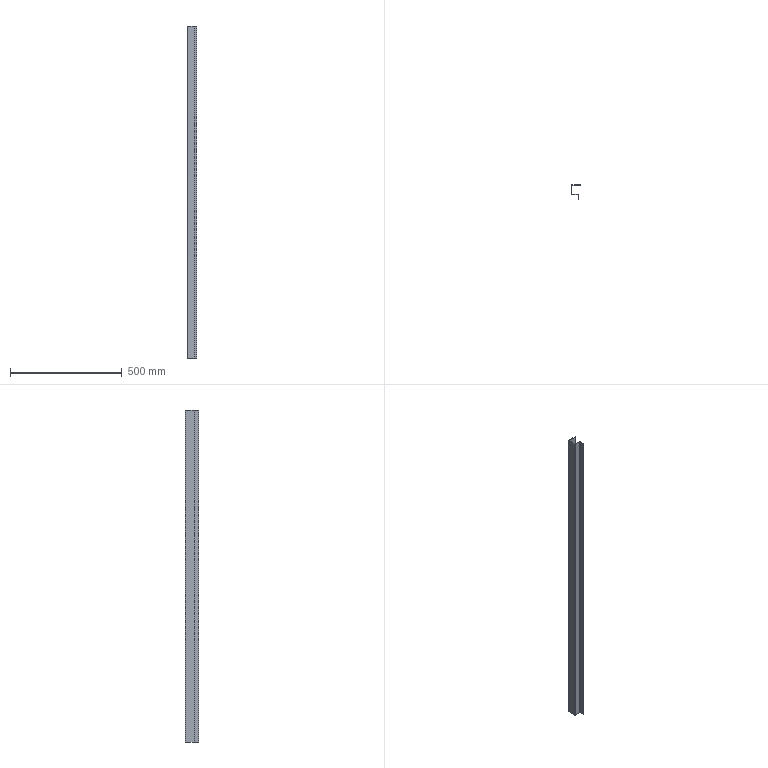Part | SolidWorks | features BaseBody 1 | 1 solid | 30 faces | box 41 x 61 x 1488 mm | volume 193542 mm3 | plane 24 | cylinder 6 | commonest cylinder face diameters 2 x3 4 x3
STEP:
#1=CARTESIAN_POINT('',(-10.,-42.,0.));
#2=VERTEX_POINT('',#1);
#3=CARTESIAN_POINT('',(-10.,-60.,0.));
#4=VERTEX_POINT('',#3);
#5=CARTESIAN_POINT('',(-10.,-40.,0.));
#6=DIRECTION('',(0.,-1.,0.));
#7=VECTOR('',#6,1000.);
#8=LINE('',#5,#7);
#9=EDGE_CURVE('',#2,#4,#8,.T.);
#10=ORIENTED_EDGE('',*,*,#9,.F.);
#11=CARTESIAN_POINT('',(-9.,-42.,0.));
#12=VERTEX_POINT('',#11);
#13=CARTESIAN_POINT('',(-10.,-42.,0.));
#14=DIRECTION('',(1.,0.,0.));
#15=VECTOR('',#14,1000.);
#16=LINE('',#13,#15);
#17=EDGE_CURVE('',#2,#12,#16,.T.);
#18=ORIENTED_EDGE('',*,*,#17,.T.);
#19=CARTESIAN_POINT('',(-9.,-60.,0.));
#20=VERTEX_POINT('',#19);
#21=CARTESIAN_POINT('',(-9.,-40.,0.));
#22=DIRECTION('',(0.,-1.,0.));
#23=VECTOR('',#22,1000.);
#24=LINE('',#21,#23);
#25=EDGE_CURVE('',#12,#20,#24,.T.);
#26=ORIENTED_EDGE('',*,*,#25,.T.);
#27=CARTESIAN_POINT('',(-9.,-60.,0.));
#28=DIRECTION('',(-1.,0.,0.));
#29=VECTOR('',#28,1000.);
#30=LINE('',#27,#29);
#31=EDGE_CURVE('',#20,#4,#30,.T.);
#32=ORIENTED_EDGE('',*,*,#31,.T.);
#33=EDGE_LOOP('',(#10,#18,#26,#32));
#34=FACE_OUTER_BOUND('',#33,.T.);
#35=CARTESIAN_POINT('',(-11.,-42.,0.));
#36=DIRECTION('',(0.,0.,1.));
#37=DIRECTION('',(1.,0.,0.));
#38=AXIS2_PLACEMENT_3D('',#35,#36,#37);
#39=PLANE('',#38);
#40=ADVANCED_FACE('',(#34),#39,.F.);
#41=CARTESIAN_POINT('',(0.,1.,1488.));
#42=VERTEX_POINT('',#41);
#43=CARTESIAN_POINT('',(-39.,1.,1488.));
#44=VERTEX_POINT('',#43);
#45=CARTESIAN_POINT('',(0.,1.,1488.));
#46=DIRECTION('',(-1.,0.,0.));
#47=VECTOR('',#46,1000.);
#48=LINE('',#45,#47);
#49=EDGE_CURVE('',#42,#44,#48,.T.);
#50=ORIENTED_EDGE('',*,*,#49,.T.);
#51=CARTESIAN_POINT('',(-39.,0.,1488.));
#52=VERTEX_POINT('',#51);
#53=CARTESIAN_POINT('',(-39.,1.,1488.));
#54=DIRECTION('',(0.,-1.,0.));
#55=VECTOR('',#54,1000.);
#56=LINE('',#53,#55);
#57=EDGE_CURVE('',#44,#52,#56,.T.);
#58=ORIENTED_EDGE('',*,*,#57,.T.);
#59=CARTESIAN_POINT('',(0.,0.,1488.));
#60=VERTEX_POINT('',#59);
#61=CARTESIAN_POINT('',(0.,0.,1488.));
#62=DIRECTION('',(-1.,0.,0.));
#63=VECTOR('',#62,1000.);
#64=LINE('',#61,#63);
#65=EDGE_CURVE('',#60,#52,#64,.T.);
#66=ORIENTED_EDGE('',*,*,#65,.F.);
#67=CARTESIAN_POINT('',(0.,1.,1488.));
#68=DIRECTION('',(0.,-1.,0.));
#69=VECTOR('',#68,1000.);
#70=LINE('',#67,#69);
#71=EDGE_CURVE('',#42,#60,#70,.T.);
#72=ORIENTED_EDGE('',*,*,#71,.F.);
#73=EDGE_LOOP('',(#50,#58,#66,#72));
#74=FACE_OUTER_BOUND('',#73,.T.);
#75=CARTESIAN_POINT('',(-11.,-42.,1488.));
#76=DIRECTION('',(0.,0.,1.));
#77=DIRECTION('',(1.,0.,0.));
#78=AXIS2_PLACEMENT_3D('',#75,#76,#77);
#79=PLANE('',#78);
#80=ADVANCED_FACE('',(#74),#79,.T.);
#81=CARTESIAN_POINT('',(-11.,-41.,0.));
#82=VERTEX_POINT('',#81);
#83=CARTESIAN_POINT('',(-11.,-42.,0.));
#84=DIRECTION('',(0.,0.,-1.));
#85=DIRECTION('',(1.,0.,0.));
#86=AXIS2_PLACEMENT_3D('',#83,#84,#85);
#87=CIRCLE('',#86,1.);
#88=EDGE_CURVE('',#82,#2,#87,.T.);
#89=ORIENTED_EDGE('',*,*,#88,.T.);
#90=CARTESIAN_POINT('',(-10.,-42.,1488.));
#91=VERTEX_POINT('',#90);
#92=CARTESIAN_POINT('',(-10.,-42.,1488.));
#93=DIRECTION('',(0.,0.,-1.));
#94=VECTOR('',#93,1000.);
#95=LINE('',#92,#94);
#96=EDGE_CURVE('',#91,#2,#95,.T.);
#97=ORIENTED_EDGE('',*,*,#96,.F.);
#98=CARTESIAN_POINT('',(-11.,-41.,1488.));
#99=VERTEX_POINT('',#98);
#100=CARTESIAN_POINT('',(-11.,-42.,1488.));
#101=DIRECTION('',(0.,0.,-1.));
#102=DIRECTION('',(1.,0.,0.));
#103=AXIS2_PLACEMENT_3D('',#100,#101,#102);
#104=CIRCLE('',#103,1.);
#105=EDGE_CURVE('',#99,#91,#104,.T.);
#106=ORIENTED_EDGE('',*,*,#105,.F.);
#107=CARTESIAN_POINT('',(-11.,-41.,1488.));
#108=DIRECTION('',(0.,0.,-1.));
#109=VECTOR('',#108,1000.);
#110=LINE('',#107,#109);
#111=EDGE_CURVE('',#99,#82,#110,.T.);
#112=ORIENTED_EDGE('',*,*,#111,.T.);
#113=EDGE_LOOP('',(#89,#97,#106,#112));
#114=FACE_OUTER_BOUND('',#113,.T.);
#115=CARTESIAN_POINT('',(-11.,-42.,1488.));
#116=DIRECTION('',(0.,0.,-1.));
#117=DIRECTION('',(-1.,0.,0.));
#118=AXIS2_PLACEMENT_3D('',#115,#116,#117);
#119=CYLINDRICAL_SURFACE('',#118,1.);
#120=ADVANCED_FACE('',(#114),#119,.F.);
#121=CARTESIAN_POINT('',(-39.,-41.,0.));
#122=VERTEX_POINT('',#121);
#123=CARTESIAN_POINT('',(-40.,-41.,0.));
#124=DIRECTION('',(1.,0.,0.));
#125=VECTOR('',#124,1000.);
#126=LINE('',#123,#125);
#127=EDGE_CURVE('',#122,#82,#126,.T.);
#128=ORIENTED_EDGE('',*,*,#127,.T.);
#129=ORIENTED_EDGE('',*,*,#111,.F.);
#130=CARTESIAN_POINT('',(-39.,-41.,1488.));
#131=VERTEX_POINT('',#130);
#132=CARTESIAN_POINT('',(-40.,-41.,1488.));
#133=DIRECTION('',(1.,0.,0.));
#134=VECTOR('',#133,1000.);
#135=LINE('',#132,#134);
#136=EDGE_CURVE('',#131,#99,#135,.T.);
#137=ORIENTED_EDGE('',*,*,#136,.F.);
#138=CARTESIAN_POINT('',(-39.,-41.,1488.));
#139=DIRECTION('',(0.,0.,-1.));
#140=VECTOR('',#139,1000.);
#141=LINE('',#138,#140);
#142=EDGE_CURVE('',#131,#122,#141,.T.);
#143=ORIENTED_EDGE('',*,*,#142,.T.);
#144=EDGE_LOOP('',(#128,#129,#137,#143));
#145=FACE_OUTER_BOUND('',#144,.T.);
#146=CARTESIAN_POINT('',(-40.,-41.,1488.));
#147=DIRECTION('',(0.,1.,0.));
#148=DIRECTION('',(1.,0.,0.));
#149=AXIS2_PLACEMENT_3D('',#146,#147,#148);
#150=PLANE('',#149);
#151=ADVANCED_FACE('',(#145),#150,.F.);
#152=CARTESIAN_POINT('',(-41.,-39.,0.));
#153=VERTEX_POINT('',#152);
#154=CARTESIAN_POINT('',(-39.,-39.,0.));
#155=DIRECTION('',(0.,0.,1.));
#156=DIRECTION('',(1.,0.,0.));
#157=AXIS2_PLACEMENT_3D('',#154,#155,#156);
#158=CIRCLE('',#157,2.);
#159=EDGE_CURVE('',#153,#122,#158,.T.);
#160=ORIENTED_EDGE('',*,*,#159,.T.);
#161=ORIENTED_EDGE('',*,*,#142,.F.);
#162=CARTESIAN_POINT('',(-41.,-39.,1488.));
#163=VERTEX_POINT('',#162);
#164=CARTESIAN_POINT('',(-39.,-39.,1488.));
#165=DIRECTION('',(0.,0.,1.));
#166=DIRECTION('',(1.,0.,0.));
#167=AXIS2_PLACEMENT_3D('',#164,#165,#166);
#168=CIRCLE('',#167,2.);
#169=EDGE_CURVE('',#163,#131,#168,.T.);
#170=ORIENTED_EDGE('',*,*,#169,.F.);
#171=CARTESIAN_POINT('',(-41.,-39.,1488.));
#172=DIRECTION('',(0.,0.,-1.));
#173=VECTOR('',#172,1000.);
#174=LINE('',#171,#173);
#175=EDGE_CURVE('',#163,#153,#174,.T.);
#176=ORIENTED_EDGE('',*,*,#175,.T.);
#177=EDGE_LOOP('',(#160,#161,#170,#176));
#178=FACE_OUTER_BOUND('',#177,.T.);
#179=CARTESIAN_POINT('',(-39.,-39.,1488.));
#180=DIRECTION('',(0.,0.,-1.));
#181=DIRECTION('',(-1.,0.,0.));
#182=AXIS2_PLACEMENT_3D('',#179,#180,#181);
#183=CYLINDRICAL_SURFACE('',#182,2.);
#184=ADVANCED_FACE('',(#178),#183,.T.);
#185=CARTESIAN_POINT('',(-41.,-1.,0.));
#186=VERTEX_POINT('',#185);
#187=CARTESIAN_POINT('',(-41.,0.,0.));
#188=DIRECTION('',(0.,-1.,0.));
#189=VECTOR('',#188,1000.);
#190=LINE('',#187,#189);
#191=EDGE_CURVE('',#186,#153,#190,.T.);
#192=ORIENTED_EDGE('',*,*,#191,.T.);
#193=ORIENTED_EDGE('',*,*,#175,.F.);
#194=CARTESIAN_POINT('',(-41.,-1.,1488.));
#195=VERTEX_POINT('',#194);
#196=CARTESIAN_POINT('',(-41.,0.,1488.));
#197=DIRECTION('',(0.,-1.,0.));
#198=VECTOR('',#197,1000.);
#199=LINE('',#196,#198);
#200=EDGE_CURVE('',#195,#163,#199,.T.);
#201=ORIENTED_EDGE('',*,*,#200,.F.);
#202=CARTESIAN_POINT('',(-41.,-1.,1488.));
#203=DIRECTION('',(0.,0.,-1.));
#204=VECTOR('',#203,1000.);
#205=LINE('',#202,#204);
#206=EDGE_CURVE('',#195,#186,#205,.T.);
#207=ORIENTED_EDGE('',*,*,#206,.T.);
#208=EDGE_LOOP('',(#192,#193,#201,#207));
#209=FACE_OUTER_BOUND('',#208,.T.);
#210=CARTESIAN_POINT('',(-41.,0.,1488.));
#211=DIRECTION('',(1.,0.,0.));
#212=DIRECTION('',(0.,1.,0.));
#213=AXIS2_PLACEMENT_3D('',#210,#211,#212);
#214=PLANE('',#213);
#215=ADVANCED_FACE('',(#209),#214,.F.);
#216=CARTESIAN_POINT('',(-39.,1.,0.));
#217=VERTEX_POINT('',#216);
#218=CARTESIAN_POINT('',(-39.,-1.,0.));
#219=DIRECTION('',(0.,0.,1.));
#220=DIRECTION('',(1.,0.,0.));
#221=AXIS2_PLACEMENT_3D('',#218,#219,#220);
#222=CIRCLE('',#221,2.);
#223=EDGE_CURVE('',#217,#186,#222,.T.);
#224=ORIENTED_EDGE('',*,*,#223,.T.);
#225=ORIENTED_EDGE('',*,*,#206,.F.);
#226=CARTESIAN_POINT('',(-39.,-1.,1488.));
#227=DIRECTION('',(0.,0.,1.));
#228=DIRECTION('',(1.,0.,0.));
#229=AXIS2_PLACEMENT_3D('',#226,#227,#228);
#230=CIRCLE('',#229,2.);
#231=EDGE_CURVE('',#44,#195,#230,.T.);
#232=ORIENTED_EDGE('',*,*,#231,.F.);
#233=CARTESIAN_POINT('',(-39.,1.,1488.));
#234=DIRECTION('',(0.,0.,-1.));
#235=VECTOR('',#234,1000.);
#236=LINE('',#233,#235);
#237=EDGE_CURVE('',#44,#217,#236,.T.);
#238=ORIENTED_EDGE('',*,*,#237,.T.);
#239=EDGE_LOOP('',(#224,#225,#232,#238));
#240=FACE_OUTER_BOUND('',#239,.T.);
#241=CARTESIAN_POINT('',(-39.,-1.,1488.));
#242=DIRECTION('',(0.,0.,-1.));
#243=DIRECTION('',(-1.,0.,0.));
#244=AXIS2_PLACEMENT_3D('',#241,#242,#243);
#245=CYLINDRICAL_SURFACE('',#244,2.);
#246=ADVANCED_FACE('',(#240),#245,.T.);
#247=CARTESIAN_POINT('',(0.,1.,0.));
#248=VERTEX_POINT('',#247);
#249=CARTESIAN_POINT('',(0.,1.,0.));
#250=DIRECTION('',(-1.,0.,0.));
#251=VECTOR('',#250,1000.);
#252=LINE('',#249,#251);
#253=EDGE_CURVE('',#248,#217,#252,.T.);
#254=ORIENTED_EDGE('',*,*,#253,.T.);
#255=ORIENTED_EDGE('',*,*,#237,.F.);
#256=ORIENTED_EDGE('',*,*,#49,.F.);
#257=CARTESIAN_POINT('',(0.,1.,1488.));
#258=DIRECTION('',(0.,0.,-1.));
#259=VECTOR('',#258,1000.);
#260=LINE('',#257,#259);
#261=EDGE_CURVE('',#42,#248,#260,.T.);
#262=ORIENTED_EDGE('',*,*,#261,.T.);
#263=EDGE_LOOP('',(#254,#255,#256,#262));
#264=FACE_OUTER_BOUND('',#263,.T.);
#265=CARTESIAN_POINT('',(0.,1.,1488.));
#266=DIRECTION('',(0.,-1.,0.));
#267=DIRECTION('',(0.,0.,-1.));
#268=AXIS2_PLACEMENT_3D('',#265,#266,#267);
#269=PLANE('',#268);
#270=ADVANCED_FACE('',(#264),#269,.F.);
#271=CARTESIAN_POINT('',(0.,0.,0.));
#272=VERTEX_POINT('',#271);
#273=CARTESIAN_POINT('',(0.,1.,0.));
#274=DIRECTION('',(0.,-1.,0.));
#275=VECTOR('',#274,1000.);
#276=LINE('',#273,#275);
#277=EDGE_CURVE('',#248,#272,#276,.T.);
#278=ORIENTED_EDGE('',*,*,#277,.F.);
#279=ORIENTED_EDGE('',*,*,#261,.F.);
#280=ORIENTED_EDGE('',*,*,#71,.T.);
#281=CARTESIAN_POINT('',(0.,0.,1488.));
#282=DIRECTION('',(0.,0.,-1.));
#283=VECTOR('',#282,1000.);
#284=LINE('',#281,#283);
#285=EDGE_CURVE('',#60,#272,#284,.T.);
#286=ORIENTED_EDGE('',*,*,#285,.T.);
#287=EDGE_LOOP('',(#278,#279,#280,#286));
#288=FACE_OUTER_BOUND('',#287,.T.);
#289=CARTESIAN_POINT('',(0.,1.,1488.));
#290=DIRECTION('',(1.,0.,0.));
#291=DIRECTION('',(0.,1.,0.));
#292=AXIS2_PLACEMENT_3D('',#289,#290,#291);
#293=PLANE('',#292);
#294=ADVANCED_FACE('',(#288),#293,.T.);
#295=CARTESIAN_POINT('',(-39.,0.,0.));
#296=VERTEX_POINT('',#295);
#297=CARTESIAN_POINT('',(0.,0.,0.));
#298=DIRECTION('',(-1.,0.,0.));
#299=VECTOR('',#298,1000.);
#300=LINE('',#297,#299);
#301=EDGE_CURVE('',#272,#296,#300,.T.);
#302=ORIENTED_EDGE('',*,*,#301,.F.);
#303=ORIENTED_EDGE('',*,*,#285,.F.);
#304=ORIENTED_EDGE('',*,*,#65,.T.);
#305=CARTESIAN_POINT('',(-39.,0.,1488.));
#306=DIRECTION('',(0.,0.,-1.));
#307=VECTOR('',#306,1000.);
#308=LINE('',#305,#307);
#309=EDGE_CURVE('',#52,#296,#308,.T.);
#310=ORIENTED_EDGE('',*,*,#309,.T.);
#311=EDGE_LOOP('',(#302,#303,#304,#310));
#312=FACE_OUTER_BOUND('',#311,.T.);
#313=CARTESIAN_POINT('',(0.,0.,1488.));
#314=DIRECTION('',(0.,-1.,0.));
#315=DIRECTION('',(0.,0.,-1.));
#316=AXIS2_PLACEMENT_3D('',#313,#314,#315);
#317=PLANE('',#316);
#318=ADVANCED_FACE('',(#312),#317,.T.);
#319=CARTESIAN_POINT('',(-40.,-1.,0.));
#320=VERTEX_POINT('',#319);
#321=CARTESIAN_POINT('',(-39.,-1.,0.));
#322=DIRECTION('',(0.,0.,1.));
#323=DIRECTION('',(-1.,0.,0.));
#324=AXIS2_PLACEMENT_3D('',#321,#322,#323);
#325=CIRCLE('',#324,1.);
#326=EDGE_CURVE('',#296,#320,#325,.T.);
#327=ORIENTED_EDGE('',*,*,#326,.F.);
#328=ORIENTED_EDGE('',*,*,#309,.F.);
#329=CARTESIAN_POINT('',(-40.,-1.,1488.));
#330=VERTEX_POINT('',#329);
#331=CARTESIAN_POINT('',(-39.,-1.,1488.));
#332=DIRECTION('',(0.,0.,1.));
#333=DIRECTION('',(-1.,0.,0.));
#334=AXIS2_PLACEMENT_3D('',#331,#332,#333);
#335=CIRCLE('',#334,1.);
#336=EDGE_CURVE('',#52,#330,#335,.T.);
#337=ORIENTED_EDGE('',*,*,#336,.T.);
#338=CARTESIAN_POINT('',(-40.,-1.,1488.));
#339=DIRECTION('',(0.,0.,-1.));
#340=VECTOR('',#339,1000.);
#341=LINE('',#338,#340);
#342=EDGE_CURVE('',#330,#320,#341,.T.);
#343=ORIENTED_EDGE('',*,*,#342,.T.);
#344=EDGE_LOOP('',(#327,#328,#337,#343));
#345=FACE_OUTER_BOUND('',#344,.T.);
#346=CARTESIAN_POINT('',(-39.,-1.,1488.));
#347=DIRECTION('',(0.,0.,-1.));
#348=DIRECTION('',(-1.,0.,0.));
#349=AXIS2_PLACEMENT_3D('',#346,#347,#348);
#350=CYLINDRICAL_SURFACE('',#349,1.);
#351=ADVANCED_FACE('',(#345),#350,.F.);
#352=CARTESIAN_POINT('',(-40.,-39.,0.));
#353=VERTEX_POINT('',#352);
#354=CARTESIAN_POINT('',(-40.,0.,0.));
#355=DIRECTION('',(0.,-1.,0.));
#356=VECTOR('',#355,1000.);
#357=LINE('',#354,#356);
#358=EDGE_CURVE('',#320,#353,#357,.T.);
#359=ORIENTED_EDGE('',*,*,#358,.F.);
#360=ORIENTED_EDGE('',*,*,#342,.F.);
#361=CARTESIAN_POINT('',(-40.,-39.,1488.));
#362=VERTEX_POINT('',#361);
#363=CARTESIAN_POINT('',(-40.,0.,1488.));
#364=DIRECTION('',(0.,-1.,0.));
#365=VECTOR('',#364,1000.);
#366=LINE('',#363,#365);
#367=EDGE_CURVE('',#330,#362,#366,.T.);
#368=ORIENTED_EDGE('',*,*,#367,.T.);
#369=CARTESIAN_POINT('',(-40.,-39.,1488.));
#370=DIRECTION('',(0.,0.,-1.));
#371=VECTOR('',#370,1000.);
#372=LINE('',#369,#371);
#373=EDGE_CURVE('',#362,#353,#372,.T.);
#374=ORIENTED_EDGE('',*,*,#373,.T.);
#375=EDGE_LOOP('',(#359,#360,#368,#374));
#376=FACE_OUTER_BOUND('',#375,.T.);
#377=CARTESIAN_POINT('',(-40.,0.,1488.));
#378=DIRECTION('',(1.,0.,0.));
#379=DIRECTION('',(0.,1.,0.));
#380=AXIS2_PLACEMENT_3D('',#377,#378,#379);
#381=PLANE('',#380);
#382=ADVANCED_FACE('',(#376),#381,.T.);
#383=CARTESIAN_POINT('',(-39.,-40.,0.));
#384=VERTEX_POINT('',#383);
#385=CARTESIAN_POINT('',(-39.,-39.,0.));
#386=DIRECTION('',(0.,0.,1.));
#387=DIRECTION('',(-1.,0.,0.));
#388=AXIS2_PLACEMENT_3D('',#385,#386,#387);
#389=CIRCLE('',#388,1.);
#390=EDGE_CURVE('',#353,#384,#389,.T.);
#391=ORIENTED_EDGE('',*,*,#390,.F.);
#392=ORIENTED_EDGE('',*,*,#373,.F.);
#393=CARTESIAN_POINT('',(-39.,-40.,1488.));
#394=VERTEX_POINT('',#393);
#395=CARTESIAN_POINT('',(-39.,-39.,1488.));
#396=DIRECTION('',(0.,0.,1.));
#397=DIRECTION('',(-1.,0.,0.));
#398=AXIS2_PLACEMENT_3D('',#395,#396,#397);
#399=CIRCLE('',#398,1.);
#400=EDGE_CURVE('',#362,#394,#399,.T.);
#401=ORIENTED_EDGE('',*,*,#400,.T.);
#402=CARTESIAN_POINT('',(-39.,-40.,1488.));
#403=DIRECTION('',(0.,0.,-1.));
#404=VECTOR('',#403,1000.);
#405=LINE('',#402,#404);
#406=EDGE_CURVE('',#394,#384,#405,.T.);
#407=ORIENTED_EDGE('',*,*,#406,.T.);
#408=EDGE_LOOP('',(#391,#392,#401,#407));
#409=FACE_OUTER_BOUND('',#408,.T.);
#410=CARTESIAN_POINT('',(-39.,-39.,1488.));
#411=DIRECTION('',(0.,0.,-1.));
#412=DIRECTION('',(-1.,0.,0.));
#413=AXIS2_PLACEMENT_3D('',#410,#411,#412);
#414=CYLINDRICAL_SURFACE('',#413,1.);
#415=ADVANCED_FACE('',(#409),#414,.F.);
#416=CARTESIAN_POINT('',(-11.,-40.,0.));
#417=VERTEX_POINT('',#416);
#418=CARTESIAN_POINT('',(-40.,-40.,0.));
#419=DIRECTION('',(1.,0.,0.));
#420=VECTOR('',#419,1000.);
#421=LINE('',#418,#420);
#422=EDGE_CURVE('',#384,#417,#421,.T.);
#423=ORIENTED_EDGE('',*,*,#422,.F.);
#424=ORIENTED_EDGE('',*,*,#406,.F.);
#425=CARTESIAN_POINT('',(-11.,-40.,1488.));
#426=VERTEX_POINT('',#425);
#427=CARTESIAN_POINT('',(-40.,-40.,1488.));
#428=DIRECTION('',(1.,0.,0.));
#429=VECTOR('',#428,1000.);
#430=LINE('',#427,#429);
#431=EDGE_CURVE('',#394,#426,#430,.T.);
#432=ORIENTED_EDGE('',*,*,#431,.T.);
#433=CARTESIAN_POINT('',(-11.,-40.,1488.));
#434=DIRECTION('',(0.,0.,-1.));
#435=VECTOR('',#434,1000.);
#436=LINE('',#433,#435);
#437=EDGE_CURVE('',#426,#417,#436,.T.);
#438=ORIENTED_EDGE('',*,*,#437,.T.);
#439=EDGE_LOOP('',(#423,#424,#432,#438));
#440=FACE_OUTER_BOUND('',#439,.T.);
#441=CARTESIAN_POINT('',(-40.,-40.,1488.));
#442=DIRECTION('',(0.,1.,0.));
#443=DIRECTION('',(1.,0.,0.));
#444=AXIS2_PLACEMENT_3D('',#441,#442,#443);
#445=PLANE('',#444);
#446=ADVANCED_FACE('',(#440),#445,.T.);
#447=CARTESIAN_POINT('',(-11.,-42.,0.));
#448=DIRECTION('',(0.,0.,-1.));
#449=DIRECTION('',(1.,0.,0.));
#450=AXIS2_PLACEMENT_3D('',#447,#448,#449);
#451=CIRCLE('',#450,2.);
#452=EDGE_CURVE('',#417,#12,#451,.T.);
#453=ORIENTED_EDGE('',*,*,#452,.F.);
#454=ORIENTED_EDGE('',*,*,#437,.F.);
#455=CARTESIAN_POINT('',(-9.,-42.,1488.));
#456=VERTEX_POINT('',#455);
#457=CARTESIAN_POINT('',(-11.,-42.,1488.));
#458=DIRECTION('',(0.,0.,-1.));
#459=DIRECTION('',(1.,0.,0.));
#460=AXIS2_PLACEMENT_3D('',#457,#458,#459);
#461=CIRCLE('',#460,2.);
#462=EDGE_CURVE('',#426,#456,#461,.T.);
#463=ORIENTED_EDGE('',*,*,#462,.T.);
#464=CARTESIAN_POINT('',(-9.,-42.,1488.));
#465=DIRECTION('',(0.,0.,-1.));
#466=VECTOR('',#465,1000.);
#467=LINE('',#464,#466);
#468=EDGE_CURVE('',#456,#12,#467,.T.);
#469=ORIENTED_EDGE('',*,*,#468,.T.);
#470=EDGE_LOOP('',(#453,#454,#463,#469));
#471=FACE_OUTER_BOUND('',#470,.T.);
#472=CARTESIAN_POINT('',(-11.,-42.,1488.));
#473=DIRECTION('',(0.,0.,-1.));
#474=DIRECTION('',(-1.,0.,0.));
#475=AXIS2_PLACEMENT_3D('',#472,#473,#474);
#476=CYLINDRICAL_SURFACE('',#475,2.);
#477=ADVANCED_FACE('',(#471),#476,.T.);
#478=ORIENTED_EDGE('',*,*,#25,.F.);
#479=ORIENTED_EDGE('',*,*,#468,.F.);
#480=CARTESIAN_POINT('',(-9.,-60.,1488.));
#481=VERTEX_POINT('',#480);
#482=CARTESIAN_POINT('',(-9.,-40.,1488.));
#483=DIRECTION('',(0.,-1.,0.));
#484=VECTOR('',#483,1000.);
#485=LINE('',#482,#484);
#486=EDGE_CURVE('',#456,#481,#485,.T.);
#487=ORIENTED_EDGE('',*,*,#486,.T.);
#488=CARTESIAN_POINT('',(-9.,-60.,1488.));
#489=DIRECTION('',(0.,0.,-1.));
#490=VECTOR('',#489,1000.);
#491=LINE('',#488,#490);
#492=EDGE_CURVE('',#481,#20,#491,.T.);
#493=ORIENTED_EDGE('',*,*,#492,.T.);
#494=EDGE_LOOP('',(#478,#479,#487,#493));
#495=FACE_OUTER_BOUND('',#494,.T.);
#496=CARTESIAN_POINT('',(-9.,-40.,1488.));
#497=DIRECTION('',(1.,0.,0.));
#498=DIRECTION('',(0.,1.,0.));
#499=AXIS2_PLACEMENT_3D('',#496,#497,#498);
#500=PLANE('',#499);
#501=ADVANCED_FACE('',(#495),#500,.T.);
#502=ORIENTED_EDGE('',*,*,#31,.F.);
#503=ORIENTED_EDGE('',*,*,#492,.F.);
#504=CARTESIAN_POINT('',(-10.,-60.,1488.));
#505=VERTEX_POINT('',#504);
#506=CARTESIAN_POINT('',(-9.,-60.,1488.));
#507=DIRECTION('',(-1.,0.,0.));
#508=VECTOR('',#507,1000.);
#509=LINE('',#506,#508);
#510=EDGE_CURVE('',#481,#505,#509,.T.);
#511=ORIENTED_EDGE('',*,*,#510,.T.);
#512=CARTESIAN_POINT('',(-10.,-60.,1488.));
#513=DIRECTION('',(0.,0.,-1.));
#514=VECTOR('',#513,1000.);
#515=LINE('',#512,#514);
#516=EDGE_CURVE('',#505,#4,#515,.T.);
#517=ORIENTED_EDGE('',*,*,#516,.T.);
#518=EDGE_LOOP('',(#502,#503,#511,#517));
#519=FACE_OUTER_BOUND('',#518,.T.);
#520=CARTESIAN_POINT('',(-9.,-60.,1488.));
#521=DIRECTION('',(0.,-1.,0.));
#522=DIRECTION('',(0.,0.,-1.));
#523=AXIS2_PLACEMENT_3D('',#520,#521,#522);
#524=PLANE('',#523);
#525=ADVANCED_FACE('',(#519),#524,.T.);
#526=ORIENTED_EDGE('',*,*,#9,.T.);
#527=ORIENTED_EDGE('',*,*,#516,.F.);
#528=CARTESIAN_POINT('',(-10.,-40.,1488.));
#529=DIRECTION('',(0.,-1.,0.));
#530=VECTOR('',#529,1000.);
#531=LINE('',#528,#530);
#532=EDGE_CURVE('',#91,#505,#531,.T.);
#533=ORIENTED_EDGE('',*,*,#532,.F.);
#534=ORIENTED_EDGE('',*,*,#96,.T.);
#535=EDGE_LOOP('',(#526,#527,#533,#534));
#536=FACE_OUTER_BOUND('',#535,.T.);
#537=CARTESIAN_POINT('',(-10.,-40.,1488.));
#538=DIRECTION('',(1.,0.,0.));
#539=DIRECTION('',(0.,1.,0.));
#540=AXIS2_PLACEMENT_3D('',#537,#538,#539);
#541=PLANE('',#540);
#542=ADVANCED_FACE('',(#536),#541,.F.);
#543=ORIENTED_EDGE('',*,*,#422,.T.);
#544=CARTESIAN_POINT('',(-11.,-40.,0.));
#545=DIRECTION('',(0.,-1.,0.));
#546=VECTOR('',#545,1000.);
#547=LINE('',#544,#546);
#548=EDGE_CURVE('',#417,#82,#547,.T.);
#549=ORIENTED_EDGE('',*,*,#548,.T.);
#550=ORIENTED_EDGE('',*,*,#127,.F.);
#551=CARTESIAN_POINT('',(-39.,-41.,0.));
#552=DIRECTION('',(0.,1.,0.));
#553=VECTOR('',#552,1000.);
#554=LINE('',#551,#553);
#555=EDGE_CURVE('',#122,#384,#554,.T.);
#556=ORIENTED_EDGE('',*,*,#555,.T.);
#557=EDGE_LOOP('',(#543,#549,#550,#556));
#558=FACE_OUTER_BOUND('',#557,.T.);
#559=CARTESIAN_POINT('',(-10.,-42.,0.));
#560=DIRECTION('',(0.,0.,-1.));
#561=DIRECTION('',(0.,-1.,0.));
#562=AXIS2_PLACEMENT_3D('',#559,#560,#561);
#563=PLANE('',#562);
#564=ADVANCED_FACE('',(#558),#563,.T.);
#565=ORIENTED_EDGE('',*,*,#548,.F.);
#566=ORIENTED_EDGE('',*,*,#452,.T.);
#567=ORIENTED_EDGE('',*,*,#17,.F.);
#568=ORIENTED_EDGE('',*,*,#88,.F.);
#569=EDGE_LOOP('',(#565,#566,#567,#568));
#570=FACE_OUTER_BOUND('',#569,.T.);
#571=CARTESIAN_POINT('',(-11.,-40.,0.));
#572=DIRECTION('',(0.,0.,-1.));
#573=DIRECTION('',(0.,-1.,0.));
#574=AXIS2_PLACEMENT_3D('',#571,#572,#573);
#575=PLANE('',#574);
#576=ADVANCED_FACE('',(#570),#575,.T.);
#577=ORIENTED_EDGE('',*,*,#486,.F.);
#578=CARTESIAN_POINT('',(-9.,-42.,1488.));
#579=DIRECTION('',(-1.,0.,0.));
#580=VECTOR('',#579,1000.);
#581=LINE('',#578,#580);
#582=EDGE_CURVE('',#456,#91,#581,.T.);
#583=ORIENTED_EDGE('',*,*,#582,.T.);
#584=ORIENTED_EDGE('',*,*,#532,.T.);
#585=ORIENTED_EDGE('',*,*,#510,.F.);
#586=EDGE_LOOP('',(#577,#583,#584,#585));
#587=FACE_OUTER_BOUND('',#586,.T.);
#588=CARTESIAN_POINT('',(-11.,-41.,1488.));
#589=DIRECTION('',(0.,0.,1.));
#590=DIRECTION('',(1.,0.,0.));
#591=AXIS2_PLACEMENT_3D('',#588,#589,#590);
#592=PLANE('',#591);
#593=ADVANCED_FACE('',(#587),#592,.T.);
#594=ORIENTED_EDGE('',*,*,#582,.F.);
#595=ORIENTED_EDGE('',*,*,#462,.F.);
#596=CARTESIAN_POINT('',(-11.,-41.,1488.));
#597=DIRECTION('',(0.,1.,0.));
#598=VECTOR('',#597,1000.);
#599=LINE('',#596,#598);
#600=EDGE_CURVE('',#99,#426,#599,.T.);
#601=ORIENTED_EDGE('',*,*,#600,.F.);
#602=ORIENTED_EDGE('',*,*,#105,.T.);
#603=EDGE_LOOP('',(#594,#595,#601,#602));
#604=FACE_OUTER_BOUND('',#603,.T.);
#605=CARTESIAN_POINT('',(-9.,-42.,1488.));
#606=DIRECTION('',(0.,0.,1.));
#607=DIRECTION('',(1.,0.,0.));
#608=AXIS2_PLACEMENT_3D('',#605,#606,#607);
#609=PLANE('',#608);
#610=ADVANCED_FACE('',(#604),#609,.T.);
#611=ORIENTED_EDGE('',*,*,#358,.T.);
#612=CARTESIAN_POINT('',(-40.,-39.,0.));
#613=DIRECTION('',(-1.,0.,0.));
#614=VECTOR('',#613,1000.);
#615=LINE('',#612,#614);
#616=EDGE_CURVE('',#353,#153,#615,.T.);
#617=ORIENTED_EDGE('',*,*,#616,.T.);
#618=ORIENTED_EDGE('',*,*,#191,.F.);
#619=CARTESIAN_POINT('',(-41.,-1.,0.));
#620=DIRECTION('',(1.,0.,0.));
#621=VECTOR('',#620,1000.);
#622=LINE('',#619,#621);
#623=EDGE_CURVE('',#186,#320,#622,.T.);
#624=ORIENTED_EDGE('',*,*,#623,.T.);
#625=EDGE_LOOP('',(#611,#617,#618,#624));
#626=FACE_OUTER_BOUND('',#625,.T.);
#627=CARTESIAN_POINT('',(-39.,-41.,0.));
#628=DIRECTION('',(0.,0.,-1.));
#629=DIRECTION('',(0.,-1.,0.));
#630=AXIS2_PLACEMENT_3D('',#627,#628,#629);
#631=PLANE('',#630);
#632=ADVANCED_FACE('',(#626),#631,.T.);
#633=ORIENTED_EDGE('',*,*,#616,.F.);
#634=ORIENTED_EDGE('',*,*,#390,.T.);
#635=ORIENTED_EDGE('',*,*,#555,.F.);
#636=ORIENTED_EDGE('',*,*,#159,.F.);
#637=EDGE_LOOP('',(#633,#634,#635,#636));
#638=FACE_OUTER_BOUND('',#637,.T.);
#639=CARTESIAN_POINT('',(-40.,-39.,0.));
#640=DIRECTION('',(0.,0.,-1.));
#641=DIRECTION('',(0.,-1.,0.));
#642=AXIS2_PLACEMENT_3D('',#639,#640,#641);
#643=PLANE('',#642);
#644=ADVANCED_FACE('',(#638),#643,.T.);
#645=ORIENTED_EDGE('',*,*,#431,.F.);
#646=CARTESIAN_POINT('',(-39.,-40.,1488.));
#647=DIRECTION('',(0.,-1.,0.));
#648=VECTOR('',#647,1000.);
#649=LINE('',#646,#648);
#650=EDGE_CURVE('',#394,#131,#649,.T.);
#651=ORIENTED_EDGE('',*,*,#650,.T.);
#652=ORIENTED_EDGE('',*,*,#136,.T.);
#653=ORIENTED_EDGE('',*,*,#600,.T.);
#654=EDGE_LOOP('',(#645,#651,#652,#653));
#655=FACE_OUTER_BOUND('',#654,.T.);
#656=CARTESIAN_POINT('',(-41.,-39.,1488.));
#657=DIRECTION('',(0.,0.,1.));
#658=DIRECTION('',(1.,0.,0.));
#659=AXIS2_PLACEMENT_3D('',#656,#657,#658);
#660=PLANE('',#659);
#661=ADVANCED_FACE('',(#655),#660,.T.);
#662=ORIENTED_EDGE('',*,*,#650,.F.);
#663=ORIENTED_EDGE('',*,*,#400,.F.);
#664=CARTESIAN_POINT('',(-41.,-39.,1488.));
#665=DIRECTION('',(1.,0.,0.));
#666=VECTOR('',#665,1000.);
#667=LINE('',#664,#666);
#668=EDGE_CURVE('',#163,#362,#667,.T.);
#669=ORIENTED_EDGE('',*,*,#668,.F.);
#670=ORIENTED_EDGE('',*,*,#169,.T.);
#671=EDGE_LOOP('',(#662,#663,#669,#670));
#672=FACE_OUTER_BOUND('',#671,.T.);
#673=CARTESIAN_POINT('',(-39.,-40.,1488.));
#674=DIRECTION('',(0.,0.,1.));
#675=DIRECTION('',(1.,0.,0.));
#676=AXIS2_PLACEMENT_3D('',#673,#674,#675);
#677=PLANE('',#676);
#678=ADVANCED_FACE('',(#672),#677,.T.);
#679=ORIENTED_EDGE('',*,*,#301,.T.);
#680=CARTESIAN_POINT('',(-39.,0.,0.));
#681=DIRECTION('',(0.,1.,0.));
#682=VECTOR('',#681,1000.);
#683=LINE('',#680,#682);
#684=EDGE_CURVE('',#296,#217,#683,.T.);
#685=ORIENTED_EDGE('',*,*,#684,.T.);
#686=ORIENTED_EDGE('',*,*,#253,.F.);
#687=ORIENTED_EDGE('',*,*,#277,.T.);
#688=EDGE_LOOP('',(#679,#685,#686,#687));
#689=FACE_OUTER_BOUND('',#688,.T.);
#690=CARTESIAN_POINT('',(-41.,-1.,0.));
#691=DIRECTION('',(0.,0.,-1.));
#692=DIRECTION('',(0.,-1.,0.));
#693=AXIS2_PLACEMENT_3D('',#690,#691,#692);
#694=PLANE('',#693);
#695=ADVANCED_FACE('',(#689),#694,.T.);
#696=ORIENTED_EDGE('',*,*,#684,.F.);
#697=ORIENTED_EDGE('',*,*,#326,.T.);
#698=ORIENTED_EDGE('',*,*,#623,.F.);
#699=ORIENTED_EDGE('',*,*,#223,.F.);
#700=EDGE_LOOP('',(#696,#697,#698,#699));
#701=FACE_OUTER_BOUND('',#700,.T.);
#702=CARTESIAN_POINT('',(-39.,0.,0.));
#703=DIRECTION('',(0.,0.,-1.));
#704=DIRECTION('',(0.,-1.,0.));
#705=AXIS2_PLACEMENT_3D('',#702,#703,#704);
#706=PLANE('',#705);
#707=ADVANCED_FACE('',(#701),#706,.T.);
#708=ORIENTED_EDGE('',*,*,#367,.F.);
#709=CARTESIAN_POINT('',(-40.,-1.,1488.));
#710=DIRECTION('',(-1.,0.,0.));
#711=VECTOR('',#710,1000.);
#712=LINE('',#709,#711);
#713=EDGE_CURVE('',#330,#195,#712,.T.);
#714=ORIENTED_EDGE('',*,*,#713,.T.);
#715=ORIENTED_EDGE('',*,*,#200,.T.);
#716=ORIENTED_EDGE('',*,*,#668,.T.);
#717=EDGE_LOOP('',(#708,#714,#715,#716));
#718=FACE_OUTER_BOUND('',#717,.T.);
#719=CARTESIAN_POINT('',(-39.,1.,1488.));
#720=DIRECTION('',(0.,0.,1.));
#721=DIRECTION('',(1.,0.,0.));
#722=AXIS2_PLACEMENT_3D('',#719,#720,#721);
#723=PLANE('',#722);
#724=ADVANCED_FACE('',(#718),#723,.T.);
#725=ORIENTED_EDGE('',*,*,#713,.F.);
#726=ORIENTED_EDGE('',*,*,#336,.F.);
#727=ORIENTED_EDGE('',*,*,#57,.F.);
#728=ORIENTED_EDGE('',*,*,#231,.T.);
#729=EDGE_LOOP('',(#725,#726,#727,#728));
#730=FACE_OUTER_BOUND('',#729,.T.);
#731=CARTESIAN_POINT('',(-40.,-1.,1488.));
#732=DIRECTION('',(0.,0.,1.));
#733=DIRECTION('',(1.,0.,0.));
#734=AXIS2_PLACEMENT_3D('',#731,#732,#733);
#735=PLANE('',#734);
#736=ADVANCED_FACE('',(#730),#735,.T.);
#737=CLOSED_SHELL('',(#40,#80,#120,#151,#184,#215,#246,#270,#294,#318,#351,#382,#415,#446,#477,#501,#525,#542,#564,#576,#593,#610,#632,#644,#661,#678,#695,#707,#724,#736));
#738=MANIFOLD_SOLID_BREP('',#737);
#739=CARTESIAN_POINT('',(0.,0.,0.));
#740=DIRECTION('',(0.,0.,1.));
#741=DIRECTION('',(1.,0.,0.));
#742=AXIS2_PLACEMENT_3D('',#739,#740,#741);
#743=(LENGTH_UNIT()NAMED_UNIT(*)SI_UNIT(.MILLI.,.METRE.));
#744=UNCERTAINTY_MEASURE_WITH_UNIT(LENGTH_MEASURE(0.00001),#743,'','');
#745=(NAMED_UNIT(*)PLANE_ANGLE_UNIT()SI_UNIT($,.RADIAN.));
#746=(NAMED_UNIT(*)SI_UNIT($,.STERADIAN.)SOLID_ANGLE_UNIT());
#747=(GEOMETRIC_REPRESENTATION_CONTEXT(3)GLOBAL_UNCERTAINTY_ASSIGNED_CONTEXT((#744))GLOBAL_UNIT_ASSIGNED_CONTEXT((#743,#745,#746))REPRESENTATION_CONTEXT('',''));
#748=ADVANCED_BREP_SHAPE_REPRESENTATION('',(#738,#742),#747);